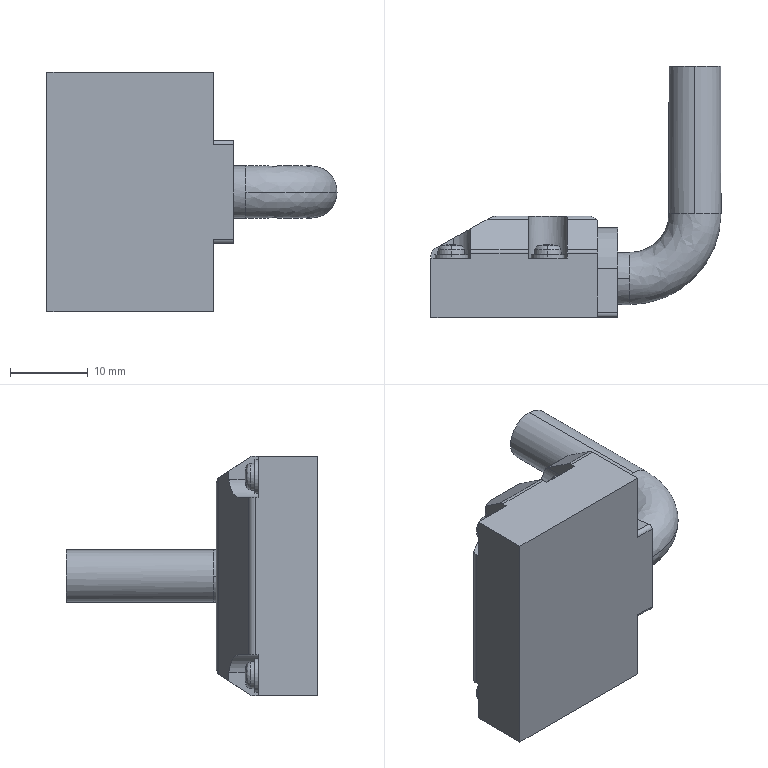Part | SolidWorks | features BaseBody 1 | 1 solid | 85 faces | box 37.25 x 32.25 x 30.8 mm | volume 9079 mm3 | cylinder 32 | plane 31 | spline 14 | cone 8 | commonest cylinder face diameters 2 x10 4.3 x8 6.7 x4 1 x3 5 x3 5.343 x2